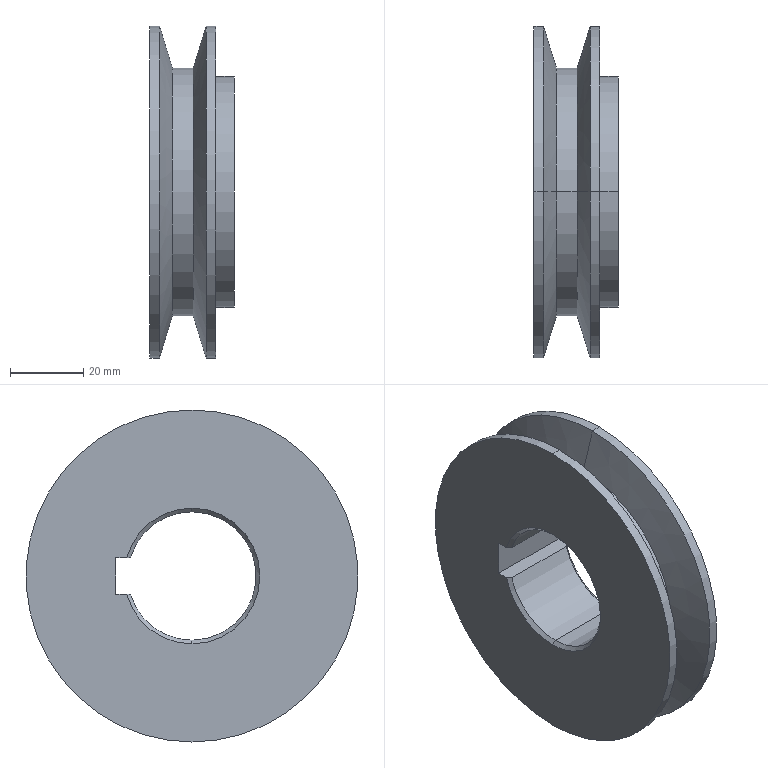Part | SolidWorks | features Chamfer 1, Cut 1, RevCut 1, Revolution 1 | 1 solid | 27 faces | box 23 x 90.5 x 90.5 mm | volume 81741 mm3 | cylinder 11 | cone 10 | plane 6 | commonest cylinder face diameters 90.5 x4 35 x3 63 x2 67.6 x2
STEP:
#1=CARTESIAN_POINT('',(1.,0.,-17.5));
#2=VERTEX_POINT('',#1);
#3=CARTESIAN_POINT('',(1.,0.,17.5));
#4=VERTEX_POINT('',#3);
#5=CARTESIAN_POINT('',(1.,0.,0.));
#6=DIRECTION('',(-1.,0.,0.));
#7=DIRECTION('',(0.,0.,-1.));
#8=AXIS2_PLACEMENT_3D('',#5,#6,#7);
#9=CIRCLE('',#8,17.5);
#10=EDGE_CURVE('',#2,#4,#9,.T.);
#11=ORIENTED_EDGE('',*,*,#10,.F.);
#12=CARTESIAN_POINT('',(0.,0.,-18.5));
#13=VERTEX_POINT('',#12);
#14=CARTESIAN_POINT('',(1.,0.,-17.5));
#15=DIRECTION('',(-0.7071,0.,-0.7071));
#16=VECTOR('',#15,1000.);
#17=LINE('',#14,#16);
#18=EDGE_CURVE('',#2,#13,#17,.T.);
#19=ORIENTED_EDGE('',*,*,#18,.T.);
#20=CARTESIAN_POINT('',(0.,0.,18.5));
#21=VERTEX_POINT('',#20);
#22=CARTESIAN_POINT('',(0.,0.,0.));
#23=DIRECTION('',(1.,0.,0.));
#24=DIRECTION('',(0.,0.,-1.));
#25=AXIS2_PLACEMENT_3D('',#22,#23,#24);
#26=CIRCLE('',#25,18.5);
#27=EDGE_CURVE('',#21,#13,#26,.T.);
#28=ORIENTED_EDGE('',*,*,#27,.F.);
#29=CARTESIAN_POINT('',(1.,0.,17.5));
#30=DIRECTION('',(-0.7071,0.,0.7071));
#31=VECTOR('',#30,1000.);
#32=LINE('',#29,#31);
#33=EDGE_CURVE('',#4,#21,#32,.T.);
#34=ORIENTED_EDGE('',*,*,#33,.F.);
#35=EDGE_LOOP('',(#11,#19,#28,#34));
#36=FACE_OUTER_BOUND('',#35,.T.);
#37=CARTESIAN_POINT('',(1.,0.,0.));
#38=DIRECTION('',(-1.,0.,0.));
#39=DIRECTION('',(0.,0.,1.));
#40=AXIS2_PLACEMENT_3D('',#37,#38,#39);
#41=CONICAL_SURFACE('',#40,17.5,0.7854);
#42=ADVANCED_FACE('',(#36),#41,.F.);
#43=CARTESIAN_POINT('',(1.,16.771,5.));
#44=VERTEX_POINT('',#43);
#45=CARTESIAN_POINT('',(1.,0.,0.));
#46=DIRECTION('',(-1.,0.,0.));
#47=DIRECTION('',(0.,0.,-1.));
#48=AXIS2_PLACEMENT_3D('',#45,#46,#47);
#49=CIRCLE('',#48,17.5);
#50=EDGE_CURVE('',#4,#44,#49,.T.);
#51=ORIENTED_EDGE('',*,*,#50,.F.);
#52=ORIENTED_EDGE('',*,*,#33,.T.);
#53=CARTESIAN_POINT('',(0.,17.812,5.));
#54=VERTEX_POINT('',#53);
#55=CARTESIAN_POINT('',(0.,0.,0.));
#56=DIRECTION('',(1.,0.,0.));
#57=DIRECTION('',(0.,0.,-1.));
#58=AXIS2_PLACEMENT_3D('',#55,#56,#57);
#59=CIRCLE('',#58,18.5);
#60=EDGE_CURVE('',#54,#21,#59,.T.);
#61=ORIENTED_EDGE('',*,*,#60,.F.);
#62=CARTESIAN_POINT('',(1.,16.771,5.));
#63=CARTESIAN_POINT('',(0.6671,17.118,5.));
#64=CARTESIAN_POINT('',(0.3337,17.465,5.));
#65=CARTESIAN_POINT('',(0.,17.812,5.));
#66=B_SPLINE_CURVE_WITH_KNOTS('',3,(#62,#63,#64,#65),.UNSPECIFIED.,.F.,.F.,(4,4),(0.002934,0.004377),.UNSPECIFIED.);
#67=EDGE_CURVE('',#44,#54,#66,.T.);
#68=ORIENTED_EDGE('',*,*,#67,.F.);
#69=EDGE_LOOP('',(#51,#52,#61,#68));
#70=FACE_OUTER_BOUND('',#69,.T.);
#71=CARTESIAN_POINT('',(1.,0.,0.));
#72=DIRECTION('',(-1.,0.,0.));
#73=DIRECTION('',(0.,0.,1.));
#74=AXIS2_PLACEMENT_3D('',#71,#72,#73);
#75=CONICAL_SURFACE('',#74,17.5,0.7854);
#76=ADVANCED_FACE('',(#70),#75,.F.);
#77=CARTESIAN_POINT('',(22.,0.,17.5));
#78=VERTEX_POINT('',#77);
#79=CARTESIAN_POINT('',(22.,0.,-17.5));
#80=VERTEX_POINT('',#79);
#81=CARTESIAN_POINT('',(22.,0.,0.));
#82=DIRECTION('',(1.,0.,0.));
#83=DIRECTION('',(0.,0.,1.));
#84=AXIS2_PLACEMENT_3D('',#81,#82,#83);
#85=CIRCLE('',#84,17.5);
#86=EDGE_CURVE('',#78,#80,#85,.T.);
#87=ORIENTED_EDGE('',*,*,#86,.F.);
#88=CARTESIAN_POINT('',(23.,0.,18.5));
#89=VERTEX_POINT('',#88);
#90=CARTESIAN_POINT('',(23.,0.,18.5));
#91=DIRECTION('',(0.7071,0.,0.7071));
#92=VECTOR('',#91,1000.);
#93=LINE('',#90,#92);
#94=EDGE_CURVE('',#78,#89,#93,.T.);
#95=ORIENTED_EDGE('',*,*,#94,.T.);
#96=CARTESIAN_POINT('',(23.,0.,-18.5));
#97=VERTEX_POINT('',#96);
#98=CARTESIAN_POINT('',(23.,0.,0.));
#99=DIRECTION('',(-1.,0.,0.));
#100=DIRECTION('',(0.,0.,1.));
#101=AXIS2_PLACEMENT_3D('',#98,#99,#100);
#102=CIRCLE('',#101,18.5);
#103=EDGE_CURVE('',#97,#89,#102,.T.);
#104=ORIENTED_EDGE('',*,*,#103,.F.);
#105=CARTESIAN_POINT('',(23.,0.,-18.5));
#106=DIRECTION('',(0.7071,0.,-0.7071));
#107=VECTOR('',#106,1000.);
#108=LINE('',#105,#107);
#109=EDGE_CURVE('',#80,#97,#108,.T.);
#110=ORIENTED_EDGE('',*,*,#109,.F.);
#111=EDGE_LOOP('',(#87,#95,#104,#110));
#112=FACE_OUTER_BOUND('',#111,.T.);
#113=CARTESIAN_POINT('',(23.,0.,0.));
#114=DIRECTION('',(1.,0.,0.));
#115=DIRECTION('',(0.,0.,-1.));
#116=AXIS2_PLACEMENT_3D('',#113,#114,#115);
#117=CONICAL_SURFACE('',#116,18.5,0.7854);
#118=ADVANCED_FACE('',(#112),#117,.F.);
#119=CARTESIAN_POINT('',(22.,16.771,-5.));
#120=VERTEX_POINT('',#119);
#121=CARTESIAN_POINT('',(22.,0.,0.));
#122=DIRECTION('',(1.,0.,0.));
#123=DIRECTION('',(0.,0.,1.));
#124=AXIS2_PLACEMENT_3D('',#121,#122,#123);
#125=CIRCLE('',#124,17.5);
#126=EDGE_CURVE('',#80,#120,#125,.T.);
#127=ORIENTED_EDGE('',*,*,#126,.F.);
#128=ORIENTED_EDGE('',*,*,#109,.T.);
#129=CARTESIAN_POINT('',(23.,17.812,-5.));
#130=VERTEX_POINT('',#129);
#131=CARTESIAN_POINT('',(23.,0.,0.));
#132=DIRECTION('',(-1.,0.,0.));
#133=DIRECTION('',(0.,0.,1.));
#134=AXIS2_PLACEMENT_3D('',#131,#132,#133);
#135=CIRCLE('',#134,18.5);
#136=EDGE_CURVE('',#130,#97,#135,.T.);
#137=ORIENTED_EDGE('',*,*,#136,.F.);
#138=CARTESIAN_POINT('',(22.,16.771,-5.));
#139=CARTESIAN_POINT('',(22.333,17.118,-5.));
#140=CARTESIAN_POINT('',(22.666,17.465,-5.));
#141=CARTESIAN_POINT('',(23.,17.812,-5.));
#142=B_SPLINE_CURVE_WITH_KNOTS('',3,(#138,#139,#140,#141),.UNSPECIFIED.,.F.,.F.,(4,4),(0.003592,0.005035),.UNSPECIFIED.);
#143=EDGE_CURVE('',#120,#130,#142,.T.);
#144=ORIENTED_EDGE('',*,*,#143,.F.);
#145=EDGE_LOOP('',(#127,#128,#137,#144));
#146=FACE_OUTER_BOUND('',#145,.T.);
#147=CARTESIAN_POINT('',(23.,0.,0.));
#148=DIRECTION('',(1.,0.,0.));
#149=DIRECTION('',(0.,0.,-1.));
#150=AXIS2_PLACEMENT_3D('',#147,#148,#149);
#151=CONICAL_SURFACE('',#150,18.5,0.7854);
#152=ADVANCED_FACE('',(#146),#151,.F.);
#153=CARTESIAN_POINT('',(6.16,0.,33.8));
#154=VERTEX_POINT('',#153);
#155=CARTESIAN_POINT('',(6.16,0.,-33.8));
#156=VERTEX_POINT('',#155);
#157=CARTESIAN_POINT('',(6.16,0.,0.));
#158=DIRECTION('',(-1.,0.,0.));
#159=DIRECTION('',(0.,0.,1.));
#160=AXIS2_PLACEMENT_3D('',#157,#158,#159);
#161=CIRCLE('',#160,33.8);
#162=EDGE_CURVE('',#154,#156,#161,.T.);
#163=ORIENTED_EDGE('',*,*,#162,.T.);
#164=CARTESIAN_POINT('',(2.659,0.,-45.25));
#165=VERTEX_POINT('',#164);
#166=CARTESIAN_POINT('',(2.659,0.,-45.25));
#167=DIRECTION('',(-0.2924,0.,-0.9563));
#168=VECTOR('',#167,1000.);
#169=LINE('',#166,#168);
#170=EDGE_CURVE('',#156,#165,#169,.T.);
#171=ORIENTED_EDGE('',*,*,#170,.T.);
#172=CARTESIAN_POINT('',(2.659,0.,45.25));
#173=VERTEX_POINT('',#172);
#174=CARTESIAN_POINT('',(2.659,0.,0.));
#175=DIRECTION('',(-1.,0.,0.));
#176=DIRECTION('',(0.,0.,1.));
#177=AXIS2_PLACEMENT_3D('',#174,#175,#176);
#178=CIRCLE('',#177,45.25);
#179=EDGE_CURVE('',#173,#165,#178,.T.);
#180=ORIENTED_EDGE('',*,*,#179,.F.);
#181=CARTESIAN_POINT('',(2.659,0.,45.25));
#182=DIRECTION('',(-0.2924,0.,0.9563));
#183=VECTOR('',#182,1000.);
#184=LINE('',#181,#183);
#185=EDGE_CURVE('',#154,#173,#184,.T.);
#186=ORIENTED_EDGE('',*,*,#185,.F.);
#187=EDGE_LOOP('',(#163,#171,#180,#186));
#188=FACE_OUTER_BOUND('',#187,.T.);
#189=CARTESIAN_POINT('',(2.659,0.,0.));
#190=DIRECTION('',(-1.,0.,0.));
#191=DIRECTION('',(0.,0.,1.));
#192=AXIS2_PLACEMENT_3D('',#189,#190,#191);
#193=CONICAL_SURFACE('',#192,45.25,1.274);
#194=ADVANCED_FACE('',(#188),#193,.T.);
#195=CARTESIAN_POINT('',(11.84,0.,33.8));
#196=VERTEX_POINT('',#195);
#197=CARTESIAN_POINT('',(11.84,0.,-33.8));
#198=VERTEX_POINT('',#197);
#199=CARTESIAN_POINT('',(11.84,0.,0.));
#200=DIRECTION('',(-1.,0.,0.));
#201=DIRECTION('',(0.,0.,1.));
#202=AXIS2_PLACEMENT_3D('',#199,#200,#201);
#203=CIRCLE('',#202,33.8);
#204=EDGE_CURVE('',#196,#198,#203,.T.);
#205=ORIENTED_EDGE('',*,*,#204,.F.);
#206=CARTESIAN_POINT('',(15.341,0.,45.25));
#207=VERTEX_POINT('',#206);
#208=CARTESIAN_POINT('',(11.84,0.,33.8));
#209=DIRECTION('',(0.2924,0.,0.9563));
#210=VECTOR('',#209,1000.);
#211=LINE('',#208,#210);
#212=EDGE_CURVE('',#196,#207,#211,.T.);
#213=ORIENTED_EDGE('',*,*,#212,.T.);
#214=CARTESIAN_POINT('',(15.341,0.,-45.25));
#215=VERTEX_POINT('',#214);
#216=CARTESIAN_POINT('',(15.341,0.,0.));
#217=DIRECTION('',(-1.,0.,0.));
#218=DIRECTION('',(0.,0.,1.));
#219=AXIS2_PLACEMENT_3D('',#216,#217,#218);
#220=CIRCLE('',#219,45.25);
#221=EDGE_CURVE('',#207,#215,#220,.T.);
#222=ORIENTED_EDGE('',*,*,#221,.T.);
#223=CARTESIAN_POINT('',(11.84,0.,-33.8));
#224=DIRECTION('',(0.2924,0.,-0.9563));
#225=VECTOR('',#224,1000.);
#226=LINE('',#223,#225);
#227=EDGE_CURVE('',#198,#215,#226,.T.);
#228=ORIENTED_EDGE('',*,*,#227,.F.);
#229=EDGE_LOOP('',(#205,#213,#222,#228));
#230=FACE_OUTER_BOUND('',#229,.T.);
#231=CARTESIAN_POINT('',(11.84,0.,0.));
#232=DIRECTION('',(1.,0.,0.));
#233=DIRECTION('',(0.,0.,-1.));
#234=AXIS2_PLACEMENT_3D('',#231,#232,#233);
#235=CONICAL_SURFACE('',#234,33.8,1.274);
#236=ADVANCED_FACE('',(#230),#235,.T.);
#237=ORIENTED_EDGE('',*,*,#204,.T.);
#238=CARTESIAN_POINT('',(0.,0.,-33.8));
#239=DIRECTION('',(-1.,0.,0.));
#240=VECTOR('',#239,1000.);
#241=LINE('',#238,#240);
#242=EDGE_CURVE('',#198,#156,#241,.T.);
#243=ORIENTED_EDGE('',*,*,#242,.T.);
#244=ORIENTED_EDGE('',*,*,#162,.F.);
#245=CARTESIAN_POINT('',(0.,0.,33.8));
#246=DIRECTION('',(-1.,0.,0.));
#247=VECTOR('',#246,1000.);
#248=LINE('',#245,#247);
#249=EDGE_CURVE('',#196,#154,#248,.T.);
#250=ORIENTED_EDGE('',*,*,#249,.F.);
#251=EDGE_LOOP('',(#237,#243,#244,#250));
#252=FACE_OUTER_BOUND('',#251,.T.);
#253=CARTESIAN_POINT('',(0.,0.,0.));
#254=DIRECTION('',(-1.,0.,0.));
#255=DIRECTION('',(0.,0.,1.));
#256=AXIS2_PLACEMENT_3D('',#253,#254,#255);
#257=CYLINDRICAL_SURFACE('',#256,33.8);
#258=ADVANCED_FACE('',(#252),#257,.T.);
#259=CARTESIAN_POINT('',(23.,0.,31.5));
#260=VERTEX_POINT('',#259);
#261=CARTESIAN_POINT('',(23.,0.,-31.5));
#262=VERTEX_POINT('',#261);
#263=CARTESIAN_POINT('',(23.,0.,0.));
#264=DIRECTION('',(-1.,0.,0.));
#265=DIRECTION('',(0.,0.,1.));
#266=AXIS2_PLACEMENT_3D('',#263,#264,#265);
#267=CIRCLE('',#266,31.5);
#268=EDGE_CURVE('',#260,#262,#267,.T.);
#269=ORIENTED_EDGE('',*,*,#268,.T.);
#270=CARTESIAN_POINT('',(18.,0.,-31.5));
#271=VERTEX_POINT('',#270);
#272=CARTESIAN_POINT('',(0.,0.,-31.5));
#273=DIRECTION('',(-1.,0.,0.));
#274=VECTOR('',#273,1000.);
#275=LINE('',#272,#274);
#276=EDGE_CURVE('',#262,#271,#275,.T.);
#277=ORIENTED_EDGE('',*,*,#276,.T.);
#278=CARTESIAN_POINT('',(18.,0.,31.5));
#279=VERTEX_POINT('',#278);
#280=CARTESIAN_POINT('',(18.,0.,0.));
#281=DIRECTION('',(-1.,0.,0.));
#282=DIRECTION('',(0.,0.,1.));
#283=AXIS2_PLACEMENT_3D('',#280,#281,#282);
#284=CIRCLE('',#283,31.5);
#285=EDGE_CURVE('',#279,#271,#284,.T.);
#286=ORIENTED_EDGE('',*,*,#285,.F.);
#287=CARTESIAN_POINT('',(0.,0.,31.5));
#288=DIRECTION('',(-1.,0.,0.));
#289=VECTOR('',#288,1000.);
#290=LINE('',#287,#289);
#291=EDGE_CURVE('',#260,#279,#290,.T.);
#292=ORIENTED_EDGE('',*,*,#291,.F.);
#293=EDGE_LOOP('',(#269,#277,#286,#292));
#294=FACE_OUTER_BOUND('',#293,.T.);
#295=CARTESIAN_POINT('',(0.,0.,0.));
#296=DIRECTION('',(-1.,0.,0.));
#297=DIRECTION('',(0.,0.,1.));
#298=AXIS2_PLACEMENT_3D('',#295,#296,#297);
#299=CYLINDRICAL_SURFACE('',#298,31.5);
#300=ADVANCED_FACE('',(#294),#299,.T.);
#301=ORIENTED_EDGE('',*,*,#86,.T.);
#302=CARTESIAN_POINT('',(0.,0.,-17.5));
#303=DIRECTION('',(-1.,0.,0.));
#304=VECTOR('',#303,1000.);
#305=LINE('',#302,#304);
#306=EDGE_CURVE('',#80,#2,#305,.T.);
#307=ORIENTED_EDGE('',*,*,#306,.T.);
#308=ORIENTED_EDGE('',*,*,#10,.T.);
#309=CARTESIAN_POINT('',(0.,0.,17.5));
#310=DIRECTION('',(-1.,0.,0.));
#311=VECTOR('',#310,1000.);
#312=LINE('',#309,#311);
#313=EDGE_CURVE('',#78,#4,#312,.T.);
#314=ORIENTED_EDGE('',*,*,#313,.F.);
#315=EDGE_LOOP('',(#301,#307,#308,#314));
#316=FACE_OUTER_BOUND('',#315,.T.);
#317=CARTESIAN_POINT('',(0.,0.,0.));
#318=DIRECTION('',(-1.,0.,0.));
#319=DIRECTION('',(0.,0.,1.));
#320=AXIS2_PLACEMENT_3D('',#317,#318,#319);
#321=CYLINDRICAL_SURFACE('',#320,17.5);
#322=ADVANCED_FACE('',(#316),#321,.F.);
#323=CARTESIAN_POINT('',(22.,16.771,5.));
#324=VERTEX_POINT('',#323);
#325=CARTESIAN_POINT('',(22.,0.,0.));
#326=DIRECTION('',(1.,0.,0.));
#327=DIRECTION('',(0.,0.,1.));
#328=AXIS2_PLACEMENT_3D('',#325,#326,#327);
#329=CIRCLE('',#328,17.5);
#330=EDGE_CURVE('',#324,#78,#329,.T.);
#331=ORIENTED_EDGE('',*,*,#330,.T.);
#332=ORIENTED_EDGE('',*,*,#313,.T.);
#333=ORIENTED_EDGE('',*,*,#50,.T.);
#334=CARTESIAN_POINT('',(23.,16.771,5.));
#335=DIRECTION('',(-1.,0.,0.));
#336=VECTOR('',#335,1000.);
#337=LINE('',#334,#336);
#338=EDGE_CURVE('',#324,#44,#337,.T.);
#339=ORIENTED_EDGE('',*,*,#338,.F.);
#340=EDGE_LOOP('',(#331,#332,#333,#339));
#341=FACE_OUTER_BOUND('',#340,.T.);
#342=CARTESIAN_POINT('',(0.,0.,0.));
#343=DIRECTION('',(-1.,0.,0.));
#344=DIRECTION('',(0.,0.,1.));
#345=AXIS2_PLACEMENT_3D('',#342,#343,#344);
#346=CYLINDRICAL_SURFACE('',#345,17.5);
#347=ADVANCED_FACE('',(#341),#346,.F.);
#348=ORIENTED_EDGE('',*,*,#179,.T.);
#349=CARTESIAN_POINT('',(0.,0.,-45.25));
#350=VERTEX_POINT('',#349);
#351=CARTESIAN_POINT('',(0.,0.,-45.25));
#352=DIRECTION('',(-1.,0.,0.));
#353=VECTOR('',#352,1000.);
#354=LINE('',#351,#353);
#355=EDGE_CURVE('',#165,#350,#354,.T.);
#356=ORIENTED_EDGE('',*,*,#355,.T.);
#357=CARTESIAN_POINT('',(0.,0.,45.25));
#358=VERTEX_POINT('',#357);
#359=CARTESIAN_POINT('',(0.,0.,0.));
#360=DIRECTION('',(-1.,0.,0.));
#361=DIRECTION('',(0.,0.,1.));
#362=AXIS2_PLACEMENT_3D('',#359,#360,#361);
#363=CIRCLE('',#362,45.25);
#364=EDGE_CURVE('',#358,#350,#363,.T.);
#365=ORIENTED_EDGE('',*,*,#364,.F.);
#366=CARTESIAN_POINT('',(0.,0.,45.25));
#367=DIRECTION('',(-1.,0.,0.));
#368=VECTOR('',#367,1000.);
#369=LINE('',#366,#368);
#370=EDGE_CURVE('',#173,#358,#369,.T.);
#371=ORIENTED_EDGE('',*,*,#370,.F.);
#372=EDGE_LOOP('',(#348,#356,#365,#371));
#373=FACE_OUTER_BOUND('',#372,.T.);
#374=CARTESIAN_POINT('',(0.,0.,0.));
#375=DIRECTION('',(-1.,0.,0.));
#376=DIRECTION('',(0.,0.,1.));
#377=AXIS2_PLACEMENT_3D('',#374,#375,#376);
#378=CYLINDRICAL_SURFACE('',#377,45.25);
#379=ADVANCED_FACE('',(#373),#378,.T.);
#380=CARTESIAN_POINT('',(18.,0.,45.25));
#381=VERTEX_POINT('',#380);
#382=CARTESIAN_POINT('',(18.,0.,-45.25));
#383=VERTEX_POINT('',#382);
#384=CARTESIAN_POINT('',(18.,0.,0.));
#385=DIRECTION('',(-1.,0.,0.));
#386=DIRECTION('',(0.,0.,1.));
#387=AXIS2_PLACEMENT_3D('',#384,#385,#386);
#388=CIRCLE('',#387,45.25);
#389=EDGE_CURVE('',#381,#383,#388,.T.);
#390=ORIENTED_EDGE('',*,*,#389,.T.);
#391=CARTESIAN_POINT('',(0.,0.,-45.25));
#392=DIRECTION('',(-1.,0.,0.));
#393=VECTOR('',#392,1000.);
#394=LINE('',#391,#393);
#395=EDGE_CURVE('',#383,#215,#394,.T.);
#396=ORIENTED_EDGE('',*,*,#395,.T.);
#397=ORIENTED_EDGE('',*,*,#221,.F.);
#398=CARTESIAN_POINT('',(0.,0.,45.25));
#399=DIRECTION('',(-1.,0.,0.));
#400=VECTOR('',#399,1000.);
#401=LINE('',#398,#400);
#402=EDGE_CURVE('',#381,#207,#401,.T.);
#403=ORIENTED_EDGE('',*,*,#402,.F.);
#404=EDGE_LOOP('',(#390,#396,#397,#403));
#405=FACE_OUTER_BOUND('',#404,.T.);
#406=CARTESIAN_POINT('',(0.,0.,0.));
#407=DIRECTION('',(-1.,0.,0.));
#408=DIRECTION('',(0.,0.,1.));
#409=AXIS2_PLACEMENT_3D('',#406,#407,#408);
#410=CYLINDRICAL_SURFACE('',#409,45.25);
#411=ADVANCED_FACE('',(#405),#410,.T.);
#412=ORIENTED_EDGE('',*,*,#395,.F.);
#413=CARTESIAN_POINT('',(18.,0.,0.));
#414=DIRECTION('',(-1.,0.,0.));
#415=DIRECTION('',(0.,0.,1.));
#416=AXIS2_PLACEMENT_3D('',#413,#414,#415);
#417=CIRCLE('',#416,45.25);
#418=EDGE_CURVE('',#383,#381,#417,.T.);
#419=ORIENTED_EDGE('',*,*,#418,.T.);
#420=ORIENTED_EDGE('',*,*,#402,.T.);
#421=CARTESIAN_POINT('',(15.341,0.,0.));
#422=DIRECTION('',(-1.,0.,0.));
#423=DIRECTION('',(0.,0.,1.));
#424=AXIS2_PLACEMENT_3D('',#421,#422,#423);
#425=CIRCLE('',#424,45.25);
#426=EDGE_CURVE('',#215,#207,#425,.T.);
#427=ORIENTED_EDGE('',*,*,#426,.F.);
#428=EDGE_LOOP('',(#412,#419,#420,#427));
#429=FACE_OUTER_BOUND('',#428,.T.);
#430=CARTESIAN_POINT('',(0.,0.,0.));
#431=DIRECTION('',(-1.,0.,0.));
#432=DIRECTION('',(0.,0.,1.));
#433=AXIS2_PLACEMENT_3D('',#430,#431,#432);
#434=CYLINDRICAL_SURFACE('',#433,45.25);
#435=ADVANCED_FACE('',(#429),#434,.T.);
#436=ORIENTED_EDGE('',*,*,#355,.F.);
#437=CARTESIAN_POINT('',(2.659,0.,0.));
#438=DIRECTION('',(-1.,0.,0.));
#439=DIRECTION('',(0.,0.,1.));
#440=AXIS2_PLACEMENT_3D('',#437,#438,#439);
#441=CIRCLE('',#440,45.25);
#442=EDGE_CURVE('',#165,#173,#441,.T.);
#443=ORIENTED_EDGE('',*,*,#442,.T.);
#444=ORIENTED_EDGE('',*,*,#370,.T.);
#445=CARTESIAN_POINT('',(0.,0.,0.));
#446=DIRECTION('',(-1.,0.,0.));
#447=DIRECTION('',(0.,0.,1.));
#448=AXIS2_PLACEMENT_3D('',#445,#446,#447);
#449=CIRCLE('',#448,45.25);
#450=EDGE_CURVE('',#350,#358,#449,.T.);
#451=ORIENTED_EDGE('',*,*,#450,.F.);
#452=EDGE_LOOP('',(#436,#443,#444,#451));
#453=FACE_OUTER_BOUND('',#452,.T.);
#454=CARTESIAN_POINT('',(0.,0.,0.));
#455=DIRECTION('',(-1.,0.,0.));
#456=DIRECTION('',(0.,0.,1.));
#457=AXIS2_PLACEMENT_3D('',#454,#455,#456);
#458=CYLINDRICAL_SURFACE('',#457,45.25);
#459=ADVANCED_FACE('',(#453),#458,.T.);
#460=ORIENTED_EDGE('',*,*,#306,.F.);
#461=ORIENTED_EDGE('',*,*,#126,.T.);
#462=CARTESIAN_POINT('',(1.,16.771,-5.));
#463=VERTEX_POINT('',#462);
#464=CARTESIAN_POINT('',(23.,16.771,-5.));
#465=DIRECTION('',(-1.,0.,0.));
#466=VECTOR('',#465,1000.);
#467=LINE('',#464,#466);
#468=EDGE_CURVE('',#120,#463,#467,.T.);
#469=ORIENTED_EDGE('',*,*,#468,.T.);
#470=CARTESIAN_POINT('',(1.,0.,0.));
#471=DIRECTION('',(-1.,0.,0.));
#472=DIRECTION('',(0.,0.,-1.));
#473=AXIS2_PLACEMENT_3D('',#470,#471,#472);
#474=CIRCLE('',#473,17.5);
#475=EDGE_CURVE('',#463,#2,#474,.T.);
#476=ORIENTED_EDGE('',*,*,#475,.T.);
#477=EDGE_LOOP('',(#460,#461,#469,#476));
#478=FACE_OUTER_BOUND('',#477,.T.);
#479=CARTESIAN_POINT('',(0.,0.,0.));
#480=DIRECTION('',(-1.,0.,0.));
#481=DIRECTION('',(0.,0.,1.));
#482=AXIS2_PLACEMENT_3D('',#479,#480,#481);
#483=CYLINDRICAL_SURFACE('',#482,17.5);
#484=ADVANCED_FACE('',(#478),#483,.F.);
#485=CARTESIAN_POINT('',(23.,20.8,5.));
#486=VERTEX_POINT('',#485);
#487=CARTESIAN_POINT('',(23.,20.8,-5.));
#488=VERTEX_POINT('',#487);
#489=CARTESIAN_POINT('',(23.,20.8,-5.));
#490=DIRECTION('',(0.,0.,-1.));
#491=VECTOR('',#490,1000.);
#492=LINE('',#489,#491);
#493=EDGE_CURVE('',#486,#488,#492,.T.);
#494=ORIENTED_EDGE('',*,*,#493,.T.);
#495=CARTESIAN_POINT('',(23.,16.771,-5.));
#496=DIRECTION('',(0.,-1.,0.));
#497=VECTOR('',#496,1000.);
#498=LINE('',#495,#497);
#499=EDGE_CURVE('',#488,#130,#498,.T.);
#500=ORIENTED_EDGE('',*,*,#499,.T.);
#501=ORIENTED_EDGE('',*,*,#136,.T.);
#502=ORIENTED_EDGE('',*,*,#103,.T.);
#503=CARTESIAN_POINT('',(23.,17.812,5.));
#504=VERTEX_POINT('',#503);
#505=CARTESIAN_POINT('',(23.,0.,0.));
#506=DIRECTION('',(-1.,0.,0.));
#507=DIRECTION('',(0.,0.,1.));
#508=AXIS2_PLACEMENT_3D('',#505,#506,#507);
#509=CIRCLE('',#508,18.5);
#510=EDGE_CURVE('',#89,#504,#509,.T.);
#511=ORIENTED_EDGE('',*,*,#510,.T.);
#512=CARTESIAN_POINT('',(23.,16.771,5.));
#513=DIRECTION('',(0.,1.,0.));
#514=VECTOR('',#513,1000.);
#515=LINE('',#512,#514);
#516=EDGE_CURVE('',#504,#486,#515,.T.);
#517=ORIENTED_EDGE('',*,*,#516,.T.);
#518=EDGE_LOOP('',(#494,#500,#501,#502,#511,#517));
#519=FACE_BOUND('',#518,.T.);
#520=ORIENTED_EDGE('',*,*,#268,.F.);
#521=CARTESIAN_POINT('',(23.,0.,0.));
#522=DIRECTION('',(-1.,0.,0.));
#523=DIRECTION('',(0.,0.,1.));
#524=AXIS2_PLACEMENT_3D('',#521,#522,#523);
#525=CIRCLE('',#524,31.5);
#526=EDGE_CURVE('',#262,#260,#525,.T.);
#527=ORIENTED_EDGE('',*,*,#526,.F.);
#528=EDGE_LOOP('',(#520,#527));
#529=FACE_OUTER_BOUND('',#528,.T.);
#530=CARTESIAN_POINT('',(23.,31.5,0.));
#531=DIRECTION('',(-1.,0.,0.));
#532=DIRECTION('',(0.,0.,1.));
#533=AXIS2_PLACEMENT_3D('',#530,#531,#532);
#534=PLANE('',#533);
#535=ADVANCED_FACE('',(#519,#529),#534,.F.);
#536=ORIENTED_EDGE('',*,*,#276,.F.);
#537=ORIENTED_EDGE('',*,*,#526,.T.);
#538=ORIENTED_EDGE('',*,*,#291,.T.);
#539=CARTESIAN_POINT('',(18.,0.,0.));
#540=DIRECTION('',(-1.,0.,0.));
#541=DIRECTION('',(0.,0.,1.));
#542=AXIS2_PLACEMENT_3D('',#539,#540,#541);
#543=CIRCLE('',#542,31.5);
#544=EDGE_CURVE('',#271,#279,#543,.T.);
#545=ORIENTED_EDGE('',*,*,#544,.F.);
#546=EDGE_LOOP('',(#536,#537,#538,#545));
#547=FACE_OUTER_BOUND('',#546,.T.);
#548=CARTESIAN_POINT('',(0.,0.,0.));
#549=DIRECTION('',(-1.,0.,0.));
#550=DIRECTION('',(0.,0.,1.));
#551=AXIS2_PLACEMENT_3D('',#548,#549,#550);
#552=CYLINDRICAL_SURFACE('',#551,31.5);
#553=ADVANCED_FACE('',(#547),#552,.T.);
#554=ORIENTED_EDGE('',*,*,#389,.F.);
#555=ORIENTED_EDGE('',*,*,#418,.F.);
#556=EDGE_LOOP('',(#554,#555));
#557=FACE_OUTER_BOUND('',#556,.T.);
#558=ORIENTED_EDGE('',*,*,#285,.T.);
#559=ORIENTED_EDGE('',*,*,#544,.T.);
#560=EDGE_LOOP('',(#558,#559));
#561=FACE_BOUND('',#560,.T.);
#562=CARTESIAN_POINT('',(18.,45.25,0.));
#563=DIRECTION('',(-1.,0.,0.));
#564=DIRECTION('',(0.,0.,1.));
#565=AXIS2_PLACEMENT_3D('',#562,#563,#564);
#566=PLANE('',#565);
#567=ADVANCED_FACE('',(#557,#561),#566,.F.);
#568=ORIENTED_EDGE('',*,*,#60,.T.);
#569=ORIENTED_EDGE('',*,*,#27,.T.);
#570=CARTESIAN_POINT('',(0.,17.812,-5.));
#571=VERTEX_POINT('',#570);
#572=CARTESIAN_POINT('',(0.,0.,0.));
#573=DIRECTION('',(1.,0.,0.));
#574=DIRECTION('',(0.,0.,-1.));
#575=AXIS2_PLACEMENT_3D('',#572,#573,#574);
#576=CIRCLE('',#575,18.5);
#577=EDGE_CURVE('',#13,#571,#576,.T.);
#578=ORIENTED_EDGE('',*,*,#577,.T.);
#579=CARTESIAN_POINT('',(0.,20.8,-5.));
#580=VERTEX_POINT('',#579);
#581=CARTESIAN_POINT('',(0.,16.771,-5.));
#582=DIRECTION('',(0.,-1.,0.));
#583=VECTOR('',#582,1000.);
#584=LINE('',#581,#583);
#585=EDGE_CURVE('',#580,#571,#584,.T.);
#586=ORIENTED_EDGE('',*,*,#585,.F.);
#587=CARTESIAN_POINT('',(0.,20.8,5.));
#588=VERTEX_POINT('',#587);
#589=CARTESIAN_POINT('',(0.,20.8,-5.));
#590=DIRECTION('',(0.,0.,-1.));
#591=VECTOR('',#590,1000.);
#592=LINE('',#589,#591);
#593=EDGE_CURVE('',#588,#580,#592,.T.);
#594=ORIENTED_EDGE('',*,*,#593,.F.);
#595=CARTESIAN_POINT('',(0.,16.771,5.));
#596=DIRECTION('',(0.,1.,0.));
#597=VECTOR('',#596,1000.);
#598=LINE('',#595,#597);
#599=EDGE_CURVE('',#54,#588,#598,.T.);
#600=ORIENTED_EDGE('',*,*,#599,.F.);
#601=EDGE_LOOP('',(#568,#569,#578,#586,#594,#600));
#602=FACE_BOUND('',#601,.T.);
#603=ORIENTED_EDGE('',*,*,#364,.T.);
#604=ORIENTED_EDGE('',*,*,#450,.T.);
#605=EDGE_LOOP('',(#603,#604));
#606=FACE_OUTER_BOUND('',#605,.T.);
#607=CARTESIAN_POINT('',(0.,17.5,0.));
#608=DIRECTION('',(1.,0.,0.));
#609=DIRECTION('',(0.,0.,-1.));
#610=AXIS2_PLACEMENT_3D('',#607,#608,#609);
#611=PLANE('',#610);
#612=ADVANCED_FACE('',(#602,#606),#611,.F.);
#613=ORIENTED_EDGE('',*,*,#242,.F.);
#614=CARTESIAN_POINT('',(11.84,0.,0.));
#615=DIRECTION('',(-1.,0.,0.));
#616=DIRECTION('',(0.,0.,1.));
#617=AXIS2_PLACEMENT_3D('',#614,#615,#616);
#618=CIRCLE('',#617,33.8);
#619=EDGE_CURVE('',#198,#196,#618,.T.);
#620=ORIENTED_EDGE('',*,*,#619,.T.);
#621=ORIENTED_EDGE('',*,*,#249,.T.);
#622=CARTESIAN_POINT('',(6.16,0.,0.));
#623=DIRECTION('',(-1.,0.,0.));
#624=DIRECTION('',(0.,0.,1.));
#625=AXIS2_PLACEMENT_3D('',#622,#623,#624);
#626=CIRCLE('',#625,33.8);
#627=EDGE_CURVE('',#156,#154,#626,.T.);
#628=ORIENTED_EDGE('',*,*,#627,.F.);
#629=EDGE_LOOP('',(#613,#620,#621,#628));
#630=FACE_OUTER_BOUND('',#629,.T.);
#631=CARTESIAN_POINT('',(0.,0.,0.));
#632=DIRECTION('',(-1.,0.,0.));
#633=DIRECTION('',(0.,0.,1.));
#634=AXIS2_PLACEMENT_3D('',#631,#632,#633);
#635=CYLINDRICAL_SURFACE('',#634,33.8);
#636=ADVANCED_FACE('',(#630),#635,.T.);
#637=ORIENTED_EDGE('',*,*,#212,.F.);
#638=ORIENTED_EDGE('',*,*,#619,.F.);
#639=ORIENTED_EDGE('',*,*,#227,.T.);
#640=ORIENTED_EDGE('',*,*,#426,.T.);
#641=EDGE_LOOP('',(#637,#638,#639,#640));
#642=FACE_OUTER_BOUND('',#641,.T.);
#643=CARTESIAN_POINT('',(11.84,0.,0.));
#644=DIRECTION('',(1.,0.,0.));
#645=DIRECTION('',(0.,0.,-1.));
#646=AXIS2_PLACEMENT_3D('',#643,#644,#645);
#647=CONICAL_SURFACE('',#646,33.8,1.274);
#648=ADVANCED_FACE('',(#642),#647,.T.);
#649=ORIENTED_EDGE('',*,*,#170,.F.);
#650=ORIENTED_EDGE('',*,*,#627,.T.);
#651=ORIENTED_EDGE('',*,*,#185,.T.);
#652=ORIENTED_EDGE('',*,*,#442,.F.);
#653=EDGE_LOOP('',(#649,#650,#651,#652));
#654=FACE_OUTER_BOUND('',#653,.T.);
#655=CARTESIAN_POINT('',(2.659,0.,0.));
#656=DIRECTION('',(-1.,0.,0.));
#657=DIRECTION('',(0.,0.,1.));
#658=AXIS2_PLACEMENT_3D('',#655,#656,#657);
#659=CONICAL_SURFACE('',#658,45.25,1.274);
#660=ADVANCED_FACE('',(#654),#659,.T.);
#661=ORIENTED_EDGE('',*,*,#94,.F.);
#662=ORIENTED_EDGE('',*,*,#330,.F.);
#663=CARTESIAN_POINT('',(23.,17.812,5.));
#664=CARTESIAN_POINT('',(22.666,17.465,5.));
#665=CARTESIAN_POINT('',(22.333,17.118,5.));
#666=CARTESIAN_POINT('',(22.,16.771,5.));
#667=B_SPLINE_CURVE_WITH_KNOTS('',3,(#663,#664,#665,#666),.UNSPECIFIED.,.F.,.F.,(4,4),(0.002806,0.00425),.UNSPECIFIED.);
#668=EDGE_CURVE('',#504,#324,#667,.T.);
#669=ORIENTED_EDGE('',*,*,#668,.F.);
#670=ORIENTED_EDGE('',*,*,#510,.F.);
#671=EDGE_LOOP('',(#661,#662,#669,#670));
#672=FACE_OUTER_BOUND('',#671,.T.);
#673=CARTESIAN_POINT('',(23.,0.,0.));
#674=DIRECTION('',(1.,0.,0.));
#675=DIRECTION('',(0.,0.,-1.));
#676=AXIS2_PLACEMENT_3D('',#673,#674,#675);
#677=CONICAL_SURFACE('',#676,18.5,0.7854);
#678=ADVANCED_FACE('',(#672),#677,.F.);
#679=ORIENTED_EDGE('',*,*,#18,.F.);
#680=ORIENTED_EDGE('',*,*,#475,.F.);
#681=CARTESIAN_POINT('',(0.,17.812,-5.));
#682=CARTESIAN_POINT('',(0.3337,17.465,-5.));
#683=CARTESIAN_POINT('',(0.6671,17.118,-5.));
#684=CARTESIAN_POINT('',(1.,16.771,-5.));
#685=B_SPLINE_CURVE_WITH_KNOTS('',3,(#681,#682,#683,#684),.UNSPECIFIED.,.F.,.F.,(4,4),(0.003465,0.004908),.UNSPECIFIED.);
#686=EDGE_CURVE('',#571,#463,#685,.T.);
#687=ORIENTED_EDGE('',*,*,#686,.F.);
#688=ORIENTED_EDGE('',*,*,#577,.F.);
#689=EDGE_LOOP('',(#679,#680,#687,#688));
#690=FACE_OUTER_BOUND('',#689,.T.);
#691=CARTESIAN_POINT('',(1.,0.,0.));
#692=DIRECTION('',(-1.,0.,0.));
#693=DIRECTION('',(0.,0.,1.));
#694=AXIS2_PLACEMENT_3D('',#691,#692,#693);
#695=CONICAL_SURFACE('',#694,17.5,0.7854);
#696=ADVANCED_FACE('',(#690),#695,.F.);
#697=ORIENTED_EDGE('',*,*,#143,.T.);
#698=ORIENTED_EDGE('',*,*,#499,.F.);
#699=CARTESIAN_POINT('',(23.,20.8,-5.));
#700=DIRECTION('',(-1.,0.,0.));
#701=VECTOR('',#700,1000.);
#702=LINE('',#699,#701);
#703=EDGE_CURVE('',#488,#580,#702,.T.);
#704=ORIENTED_EDGE('',*,*,#703,.T.);
#705=ORIENTED_EDGE('',*,*,#585,.T.);
#706=ORIENTED_EDGE('',*,*,#686,.T.);
#707=ORIENTED_EDGE('',*,*,#468,.F.);
#708=EDGE_LOOP('',(#697,#698,#704,#705,#706,#707));
#709=FACE_OUTER_BOUND('',#708,.T.);
#710=CARTESIAN_POINT('',(23.,16.771,-5.));
#711=DIRECTION('',(0.,0.,-1.));
#712=DIRECTION('',(-1.,0.,0.));
#713=AXIS2_PLACEMENT_3D('',#710,#711,#712);
#714=PLANE('',#713);
#715=ADVANCED_FACE('',(#709),#714,.F.);
#716=ORIENTED_EDGE('',*,*,#593,.T.);
#717=ORIENTED_EDGE('',*,*,#703,.F.);
#718=ORIENTED_EDGE('',*,*,#493,.F.);
#719=CARTESIAN_POINT('',(23.,20.8,5.));
#720=DIRECTION('',(-1.,0.,0.));
#721=VECTOR('',#720,1000.);
#722=LINE('',#719,#721);
#723=EDGE_CURVE('',#486,#588,#722,.T.);
#724=ORIENTED_EDGE('',*,*,#723,.T.);
#725=EDGE_LOOP('',(#716,#717,#718,#724));
#726=FACE_OUTER_BOUND('',#725,.T.);
#727=CARTESIAN_POINT('',(23.,20.8,-5.));
#728=DIRECTION('',(0.,1.,0.));
#729=DIRECTION('',(0.,0.,1.));
#730=AXIS2_PLACEMENT_3D('',#727,#728,#729);
#731=PLANE('',#730);
#732=ADVANCED_FACE('',(#726),#731,.F.);
#733=ORIENTED_EDGE('',*,*,#668,.T.);
#734=ORIENTED_EDGE('',*,*,#338,.T.);
#735=ORIENTED_EDGE('',*,*,#67,.T.);
#736=ORIENTED_EDGE('',*,*,#599,.T.);
#737=ORIENTED_EDGE('',*,*,#723,.F.);
#738=ORIENTED_EDGE('',*,*,#516,.F.);
#739=EDGE_LOOP('',(#733,#734,#735,#736,#737,#738));
#740=FACE_OUTER_BOUND('',#739,.T.);
#741=CARTESIAN_POINT('',(23.,16.771,5.));
#742=DIRECTION('',(0.,0.,1.));
#743=DIRECTION('',(1.,0.,0.));
#744=AXIS2_PLACEMENT_3D('',#741,#742,#743);
#745=PLANE('',#744);
#746=ADVANCED_FACE('',(#740),#745,.F.);
#747=CLOSED_SHELL('',(#42,#76,#118,#152,#194,#236,#258,#300,#322,#347,#379,#411,#435,#459,#484,#535,#553,#567,#612,#636,#648,#660,#678,#696,#715,#732,#746));
#748=MANIFOLD_SOLID_BREP('',#747);
#749=CARTESIAN_POINT('',(0.,0.,0.));
#750=DIRECTION('',(0.,0.,1.));
#751=DIRECTION('',(1.,0.,0.));
#752=AXIS2_PLACEMENT_3D('',#749,#750,#751);
#753=(LENGTH_UNIT()NAMED_UNIT(*)SI_UNIT(.MILLI.,.METRE.));
#754=UNCERTAINTY_MEASURE_WITH_UNIT(LENGTH_MEASURE(0.00001),#753,'','');
#755=(NAMED_UNIT(*)PLANE_ANGLE_UNIT()SI_UNIT($,.RADIAN.));
#756=(NAMED_UNIT(*)SI_UNIT($,.STERADIAN.)SOLID_ANGLE_UNIT());
#757=(GEOMETRIC_REPRESENTATION_CONTEXT(3)GLOBAL_UNCERTAINTY_ASSIGNED_CONTEXT((#754))GLOBAL_UNIT_ASSIGNED_CONTEXT((#753,#755,#756))REPRESENTATION_CONTEXT('',''));
#758=ADVANCED_BREP_SHAPE_REPRESENTATION('',(#748,#752),#757);